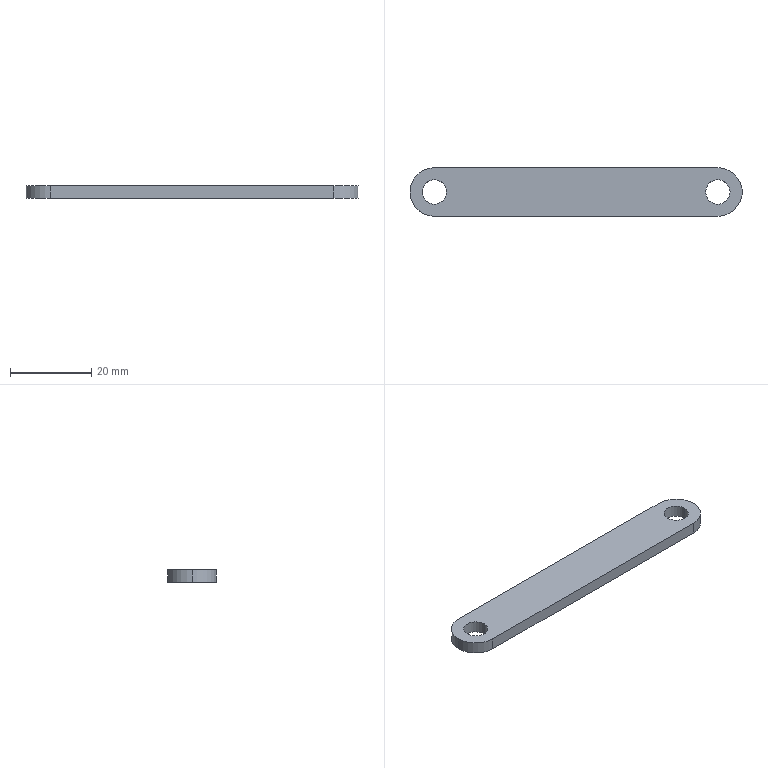Part | SolidWorks | features Extrusion 1 | 1 solid | 11 faces | box 82 x 12 x 3 mm | volume 2690 mm3 | cylinder 7 | plane 4 | commonest cylinder face diameters 6 x4 12 x3
STEP:
#1=CARTESIAN_POINT('',(67.,0.,3.));
#2=VERTEX_POINT('',#1);
#3=CARTESIAN_POINT('',(73.,0.,3.));
#4=VERTEX_POINT('',#3);
#5=CARTESIAN_POINT('',(70.,0.,3.));
#6=DIRECTION('',(0.,0.,1.));
#7=DIRECTION('',(1.,0.,0.));
#8=AXIS2_PLACEMENT_3D('',#5,#6,#7);
#9=CIRCLE('',#8,3.);
#10=EDGE_CURVE('',#2,#4,#9,.T.);
#11=ORIENTED_EDGE('',*,*,#10,.T.);
#12=CARTESIAN_POINT('',(73.,0.,0.));
#13=VERTEX_POINT('',#12);
#14=CARTESIAN_POINT('',(73.,0.,3.));
#15=DIRECTION('',(0.,0.,-1.));
#16=VECTOR('',#15,1000.);
#17=LINE('',#14,#16);
#18=EDGE_CURVE('',#4,#13,#17,.T.);
#19=ORIENTED_EDGE('',*,*,#18,.T.);
#20=CARTESIAN_POINT('',(67.,0.,0.));
#21=VERTEX_POINT('',#20);
#22=CARTESIAN_POINT('',(70.,0.,0.));
#23=DIRECTION('',(0.,0.,1.));
#24=DIRECTION('',(1.,0.,0.));
#25=AXIS2_PLACEMENT_3D('',#22,#23,#24);
#26=CIRCLE('',#25,3.);
#27=EDGE_CURVE('',#21,#13,#26,.T.);
#28=ORIENTED_EDGE('',*,*,#27,.F.);
#29=CARTESIAN_POINT('',(67.,0.,3.));
#30=DIRECTION('',(0.,0.,-1.));
#31=VECTOR('',#30,1000.);
#32=LINE('',#29,#31);
#33=EDGE_CURVE('',#2,#21,#32,.T.);
#34=ORIENTED_EDGE('',*,*,#33,.F.);
#35=EDGE_LOOP('',(#11,#19,#28,#34));
#36=FACE_OUTER_BOUND('',#35,.T.);
#37=CARTESIAN_POINT('',(70.,0.,3.));
#38=DIRECTION('',(0.,0.,-1.));
#39=DIRECTION('',(-1.,0.,0.));
#40=AXIS2_PLACEMENT_3D('',#37,#38,#39);
#41=CYLINDRICAL_SURFACE('',#40,3.);
#42=ADVANCED_FACE('',(#36),#41,.F.);
#43=CARTESIAN_POINT('',(-3.,0.,3.));
#44=VERTEX_POINT('',#43);
#45=CARTESIAN_POINT('',(3.,0.,3.));
#46=VERTEX_POINT('',#45);
#47=CARTESIAN_POINT('',(0.,0.,3.));
#48=DIRECTION('',(0.,0.,1.));
#49=DIRECTION('',(1.,0.,0.));
#50=AXIS2_PLACEMENT_3D('',#47,#48,#49);
#51=CIRCLE('',#50,3.);
#52=EDGE_CURVE('',#44,#46,#51,.T.);
#53=ORIENTED_EDGE('',*,*,#52,.T.);
#54=CARTESIAN_POINT('',(3.,0.,0.));
#55=VERTEX_POINT('',#54);
#56=CARTESIAN_POINT('',(3.,0.,3.));
#57=DIRECTION('',(0.,0.,-1.));
#58=VECTOR('',#57,1000.);
#59=LINE('',#56,#58);
#60=EDGE_CURVE('',#46,#55,#59,.T.);
#61=ORIENTED_EDGE('',*,*,#60,.T.);
#62=CARTESIAN_POINT('',(-3.,0.,0.));
#63=VERTEX_POINT('',#62);
#64=CARTESIAN_POINT('',(0.,0.,0.));
#65=DIRECTION('',(0.,0.,1.));
#66=DIRECTION('',(1.,0.,0.));
#67=AXIS2_PLACEMENT_3D('',#64,#65,#66);
#68=CIRCLE('',#67,3.);
#69=EDGE_CURVE('',#63,#55,#68,.T.);
#70=ORIENTED_EDGE('',*,*,#69,.F.);
#71=CARTESIAN_POINT('',(-3.,0.,3.));
#72=DIRECTION('',(0.,0.,-1.));
#73=VECTOR('',#72,1000.);
#74=LINE('',#71,#73);
#75=EDGE_CURVE('',#44,#63,#74,.T.);
#76=ORIENTED_EDGE('',*,*,#75,.F.);
#77=EDGE_LOOP('',(#53,#61,#70,#76));
#78=FACE_OUTER_BOUND('',#77,.T.);
#79=CARTESIAN_POINT('',(0.,0.,3.));
#80=DIRECTION('',(0.,0.,-1.));
#81=DIRECTION('',(-1.,0.,0.));
#82=AXIS2_PLACEMENT_3D('',#79,#80,#81);
#83=CYLINDRICAL_SURFACE('',#82,3.);
#84=ADVANCED_FACE('',(#78),#83,.F.);
#85=CARTESIAN_POINT('',(-6.,0.,3.));
#86=VERTEX_POINT('',#85);
#87=CARTESIAN_POINT('',(0.,-6.,3.));
#88=VERTEX_POINT('',#87);
#89=CARTESIAN_POINT('',(0.,0.,3.));
#90=DIRECTION('',(0.,0.,1.));
#91=DIRECTION('',(1.,0.,0.));
#92=AXIS2_PLACEMENT_3D('',#89,#90,#91);
#93=CIRCLE('',#92,6.);
#94=EDGE_CURVE('',#86,#88,#93,.T.);
#95=ORIENTED_EDGE('',*,*,#94,.F.);
#96=CARTESIAN_POINT('',(-6.,0.,0.));
#97=VERTEX_POINT('',#96);
#98=CARTESIAN_POINT('',(-6.,0.,3.));
#99=DIRECTION('',(0.,0.,-1.));
#100=VECTOR('',#99,1000.);
#101=LINE('',#98,#100);
#102=EDGE_CURVE('',#86,#97,#101,.T.);
#103=ORIENTED_EDGE('',*,*,#102,.T.);
#104=CARTESIAN_POINT('',(0.,-6.,0.));
#105=VERTEX_POINT('',#104);
#106=CARTESIAN_POINT('',(0.,0.,0.));
#107=DIRECTION('',(0.,0.,1.));
#108=DIRECTION('',(1.,0.,0.));
#109=AXIS2_PLACEMENT_3D('',#106,#107,#108);
#110=CIRCLE('',#109,6.);
#111=EDGE_CURVE('',#97,#105,#110,.T.);
#112=ORIENTED_EDGE('',*,*,#111,.T.);
#113=CARTESIAN_POINT('',(0.,-6.,3.));
#114=DIRECTION('',(0.,0.,-1.));
#115=VECTOR('',#114,1000.);
#116=LINE('',#113,#115);
#117=EDGE_CURVE('',#88,#105,#116,.T.);
#118=ORIENTED_EDGE('',*,*,#117,.F.);
#119=EDGE_LOOP('',(#95,#103,#112,#118));
#120=FACE_OUTER_BOUND('',#119,.T.);
#121=CARTESIAN_POINT('',(0.,0.,3.));
#122=DIRECTION('',(0.,0.,-1.));
#123=DIRECTION('',(-1.,0.,0.));
#124=AXIS2_PLACEMENT_3D('',#121,#122,#123);
#125=CYLINDRICAL_SURFACE('',#124,6.);
#126=ADVANCED_FACE('',(#120),#125,.T.);
#127=ORIENTED_EDGE('',*,*,#52,.F.);
#128=CARTESIAN_POINT('',(0.,0.,3.));
#129=DIRECTION('',(0.,0.,1.));
#130=DIRECTION('',(1.,0.,0.));
#131=AXIS2_PLACEMENT_3D('',#128,#129,#130);
#132=CIRCLE('',#131,3.);
#133=EDGE_CURVE('',#46,#44,#132,.T.);
#134=ORIENTED_EDGE('',*,*,#133,.F.);
#135=EDGE_LOOP('',(#127,#134));
#136=FACE_BOUND('',#135,.T.);
#137=CARTESIAN_POINT('',(0.,6.,3.));
#138=VERTEX_POINT('',#137);
#139=CARTESIAN_POINT('',(0.,0.,3.));
#140=DIRECTION('',(0.,0.,1.));
#141=DIRECTION('',(1.,0.,0.));
#142=AXIS2_PLACEMENT_3D('',#139,#140,#141);
#143=CIRCLE('',#142,6.);
#144=EDGE_CURVE('',#138,#86,#143,.T.);
#145=ORIENTED_EDGE('',*,*,#144,.T.);
#146=ORIENTED_EDGE('',*,*,#94,.T.);
#147=CARTESIAN_POINT('',(70.,-6.,3.));
#148=VERTEX_POINT('',#147);
#149=CARTESIAN_POINT('',(0.,-6.,3.));
#150=DIRECTION('',(1.,0.,0.));
#151=VECTOR('',#150,1000.);
#152=LINE('',#149,#151);
#153=EDGE_CURVE('',#88,#148,#152,.T.);
#154=ORIENTED_EDGE('',*,*,#153,.T.);
#155=CARTESIAN_POINT('',(70.,6.,3.));
#156=VERTEX_POINT('',#155);
#157=CARTESIAN_POINT('',(70.,0.,3.));
#158=DIRECTION('',(0.,0.,1.));
#159=DIRECTION('',(1.,0.,0.));
#160=AXIS2_PLACEMENT_3D('',#157,#158,#159);
#161=CIRCLE('',#160,6.);
#162=EDGE_CURVE('',#148,#156,#161,.T.);
#163=ORIENTED_EDGE('',*,*,#162,.T.);
#164=CARTESIAN_POINT('',(0.,6.,3.));
#165=DIRECTION('',(-1.,0.,0.));
#166=VECTOR('',#165,1000.);
#167=LINE('',#164,#166);
#168=EDGE_CURVE('',#156,#138,#167,.T.);
#169=ORIENTED_EDGE('',*,*,#168,.T.);
#170=EDGE_LOOP('',(#145,#146,#154,#163,#169));
#171=FACE_OUTER_BOUND('',#170,.T.);
#172=ORIENTED_EDGE('',*,*,#10,.F.);
#173=CARTESIAN_POINT('',(70.,0.,3.));
#174=DIRECTION('',(0.,0.,1.));
#175=DIRECTION('',(1.,0.,0.));
#176=AXIS2_PLACEMENT_3D('',#173,#174,#175);
#177=CIRCLE('',#176,3.);
#178=EDGE_CURVE('',#4,#2,#177,.T.);
#179=ORIENTED_EDGE('',*,*,#178,.F.);
#180=EDGE_LOOP('',(#172,#179));
#181=FACE_BOUND('',#180,.T.);
#182=CARTESIAN_POINT('',(0.,0.,3.));
#183=DIRECTION('',(0.,0.,1.));
#184=DIRECTION('',(1.,0.,0.));
#185=AXIS2_PLACEMENT_3D('',#182,#183,#184);
#186=PLANE('',#185);
#187=ADVANCED_FACE('',(#136,#171,#181),#186,.T.);
#188=CARTESIAN_POINT('',(0.,6.,0.));
#189=VERTEX_POINT('',#188);
#190=CARTESIAN_POINT('',(0.,0.,0.));
#191=DIRECTION('',(0.,0.,1.));
#192=DIRECTION('',(1.,0.,0.));
#193=AXIS2_PLACEMENT_3D('',#190,#191,#192);
#194=CIRCLE('',#193,6.);
#195=EDGE_CURVE('',#189,#97,#194,.T.);
#196=ORIENTED_EDGE('',*,*,#195,.F.);
#197=CARTESIAN_POINT('',(70.,6.,0.));
#198=VERTEX_POINT('',#197);
#199=CARTESIAN_POINT('',(0.,6.,0.));
#200=DIRECTION('',(-1.,0.,0.));
#201=VECTOR('',#200,1000.);
#202=LINE('',#199,#201);
#203=EDGE_CURVE('',#198,#189,#202,.T.);
#204=ORIENTED_EDGE('',*,*,#203,.F.);
#205=CARTESIAN_POINT('',(70.,-6.,0.));
#206=VERTEX_POINT('',#205);
#207=CARTESIAN_POINT('',(70.,0.,0.));
#208=DIRECTION('',(0.,0.,1.));
#209=DIRECTION('',(1.,0.,0.));
#210=AXIS2_PLACEMENT_3D('',#207,#208,#209);
#211=CIRCLE('',#210,6.);
#212=EDGE_CURVE('',#206,#198,#211,.T.);
#213=ORIENTED_EDGE('',*,*,#212,.F.);
#214=CARTESIAN_POINT('',(0.,-6.,0.));
#215=DIRECTION('',(1.,0.,0.));
#216=VECTOR('',#215,1000.);
#217=LINE('',#214,#216);
#218=EDGE_CURVE('',#105,#206,#217,.T.);
#219=ORIENTED_EDGE('',*,*,#218,.F.);
#220=ORIENTED_EDGE('',*,*,#111,.F.);
#221=EDGE_LOOP('',(#196,#204,#213,#219,#220));
#222=FACE_OUTER_BOUND('',#221,.T.);
#223=ORIENTED_EDGE('',*,*,#69,.T.);
#224=CARTESIAN_POINT('',(0.,0.,0.));
#225=DIRECTION('',(0.,0.,1.));
#226=DIRECTION('',(1.,0.,0.));
#227=AXIS2_PLACEMENT_3D('',#224,#225,#226);
#228=CIRCLE('',#227,3.);
#229=EDGE_CURVE('',#55,#63,#228,.T.);
#230=ORIENTED_EDGE('',*,*,#229,.T.);
#231=EDGE_LOOP('',(#223,#230));
#232=FACE_BOUND('',#231,.T.);
#233=ORIENTED_EDGE('',*,*,#27,.T.);
#234=CARTESIAN_POINT('',(70.,0.,0.));
#235=DIRECTION('',(0.,0.,1.));
#236=DIRECTION('',(1.,0.,0.));
#237=AXIS2_PLACEMENT_3D('',#234,#235,#236);
#238=CIRCLE('',#237,3.);
#239=EDGE_CURVE('',#13,#21,#238,.T.);
#240=ORIENTED_EDGE('',*,*,#239,.T.);
#241=EDGE_LOOP('',(#233,#240));
#242=FACE_BOUND('',#241,.T.);
#243=CARTESIAN_POINT('',(0.,0.,0.));
#244=DIRECTION('',(0.,0.,1.));
#245=DIRECTION('',(1.,0.,0.));
#246=AXIS2_PLACEMENT_3D('',#243,#244,#245);
#247=PLANE('',#246);
#248=ADVANCED_FACE('',(#222,#232,#242),#247,.F.);
#249=ORIENTED_EDGE('',*,*,#102,.F.);
#250=ORIENTED_EDGE('',*,*,#144,.F.);
#251=CARTESIAN_POINT('',(0.,6.,3.));
#252=DIRECTION('',(0.,0.,-1.));
#253=VECTOR('',#252,1000.);
#254=LINE('',#251,#253);
#255=EDGE_CURVE('',#138,#189,#254,.T.);
#256=ORIENTED_EDGE('',*,*,#255,.T.);
#257=ORIENTED_EDGE('',*,*,#195,.T.);
#258=EDGE_LOOP('',(#249,#250,#256,#257));
#259=FACE_OUTER_BOUND('',#258,.T.);
#260=CARTESIAN_POINT('',(0.,0.,3.));
#261=DIRECTION('',(0.,0.,-1.));
#262=DIRECTION('',(-1.,0.,0.));
#263=AXIS2_PLACEMENT_3D('',#260,#261,#262);
#264=CYLINDRICAL_SURFACE('',#263,6.);
#265=ADVANCED_FACE('',(#259),#264,.T.);
#266=ORIENTED_EDGE('',*,*,#218,.T.);
#267=CARTESIAN_POINT('',(70.,-6.,3.));
#268=DIRECTION('',(0.,0.,-1.));
#269=VECTOR('',#268,1000.);
#270=LINE('',#267,#269);
#271=EDGE_CURVE('',#148,#206,#270,.T.);
#272=ORIENTED_EDGE('',*,*,#271,.F.);
#273=ORIENTED_EDGE('',*,*,#153,.F.);
#274=ORIENTED_EDGE('',*,*,#117,.T.);
#275=EDGE_LOOP('',(#266,#272,#273,#274));
#276=FACE_OUTER_BOUND('',#275,.T.);
#277=CARTESIAN_POINT('',(0.,-6.,3.));
#278=DIRECTION('',(0.,1.,0.));
#279=DIRECTION('',(0.,0.,1.));
#280=AXIS2_PLACEMENT_3D('',#277,#278,#279);
#281=PLANE('',#280);
#282=ADVANCED_FACE('',(#276),#281,.F.);
#283=ORIENTED_EDGE('',*,*,#212,.T.);
#284=CARTESIAN_POINT('',(70.,6.,3.));
#285=DIRECTION('',(0.,0.,-1.));
#286=VECTOR('',#285,1000.);
#287=LINE('',#284,#286);
#288=EDGE_CURVE('',#156,#198,#287,.T.);
#289=ORIENTED_EDGE('',*,*,#288,.F.);
#290=ORIENTED_EDGE('',*,*,#162,.F.);
#291=ORIENTED_EDGE('',*,*,#271,.T.);
#292=EDGE_LOOP('',(#283,#289,#290,#291));
#293=FACE_OUTER_BOUND('',#292,.T.);
#294=CARTESIAN_POINT('',(70.,0.,3.));
#295=DIRECTION('',(0.,0.,-1.));
#296=DIRECTION('',(-1.,0.,0.));
#297=AXIS2_PLACEMENT_3D('',#294,#295,#296);
#298=CYLINDRICAL_SURFACE('',#297,6.);
#299=ADVANCED_FACE('',(#293),#298,.T.);
#300=ORIENTED_EDGE('',*,*,#203,.T.);
#301=ORIENTED_EDGE('',*,*,#255,.F.);
#302=ORIENTED_EDGE('',*,*,#168,.F.);
#303=ORIENTED_EDGE('',*,*,#288,.T.);
#304=EDGE_LOOP('',(#300,#301,#302,#303));
#305=FACE_OUTER_BOUND('',#304,.T.);
#306=CARTESIAN_POINT('',(0.,6.,3.));
#307=DIRECTION('',(0.,-1.,0.));
#308=DIRECTION('',(0.,0.,-1.));
#309=AXIS2_PLACEMENT_3D('',#306,#307,#308);
#310=PLANE('',#309);
#311=ADVANCED_FACE('',(#305),#310,.F.);
#312=ORIENTED_EDGE('',*,*,#60,.F.);
#313=ORIENTED_EDGE('',*,*,#133,.T.);
#314=ORIENTED_EDGE('',*,*,#75,.T.);
#315=ORIENTED_EDGE('',*,*,#229,.F.);
#316=EDGE_LOOP('',(#312,#313,#314,#315));
#317=FACE_OUTER_BOUND('',#316,.T.);
#318=CARTESIAN_POINT('',(0.,0.,3.));
#319=DIRECTION('',(0.,0.,-1.));
#320=DIRECTION('',(-1.,0.,0.));
#321=AXIS2_PLACEMENT_3D('',#318,#319,#320);
#322=CYLINDRICAL_SURFACE('',#321,3.);
#323=ADVANCED_FACE('',(#317),#322,.F.);
#324=ORIENTED_EDGE('',*,*,#18,.F.);
#325=ORIENTED_EDGE('',*,*,#178,.T.);
#326=ORIENTED_EDGE('',*,*,#33,.T.);
#327=ORIENTED_EDGE('',*,*,#239,.F.);
#328=EDGE_LOOP('',(#324,#325,#326,#327));
#329=FACE_OUTER_BOUND('',#328,.T.);
#330=CARTESIAN_POINT('',(70.,0.,3.));
#331=DIRECTION('',(0.,0.,-1.));
#332=DIRECTION('',(-1.,0.,0.));
#333=AXIS2_PLACEMENT_3D('',#330,#331,#332);
#334=CYLINDRICAL_SURFACE('',#333,3.);
#335=ADVANCED_FACE('',(#329),#334,.F.);
#336=CLOSED_SHELL('',(#42,#84,#126,#187,#248,#265,#282,#299,#311,#323,#335));
#337=MANIFOLD_SOLID_BREP('',#336);
#338=CARTESIAN_POINT('',(0.,0.,0.));
#339=DIRECTION('',(0.,0.,1.));
#340=DIRECTION('',(1.,0.,0.));
#341=AXIS2_PLACEMENT_3D('',#338,#339,#340);
#342=(LENGTH_UNIT()NAMED_UNIT(*)SI_UNIT(.MILLI.,.METRE.));
#343=UNCERTAINTY_MEASURE_WITH_UNIT(LENGTH_MEASURE(0.00001),#342,'','');
#344=(NAMED_UNIT(*)PLANE_ANGLE_UNIT()SI_UNIT($,.RADIAN.));
#345=(NAMED_UNIT(*)SI_UNIT($,.STERADIAN.)SOLID_ANGLE_UNIT());
#346=(GEOMETRIC_REPRESENTATION_CONTEXT(3)GLOBAL_UNCERTAINTY_ASSIGNED_CONTEXT((#343))GLOBAL_UNIT_ASSIGNED_CONTEXT((#342,#344,#345))REPRESENTATION_CONTEXT('',''));
#347=ADVANCED_BREP_SHAPE_REPRESENTATION('',(#337,#341),#346);